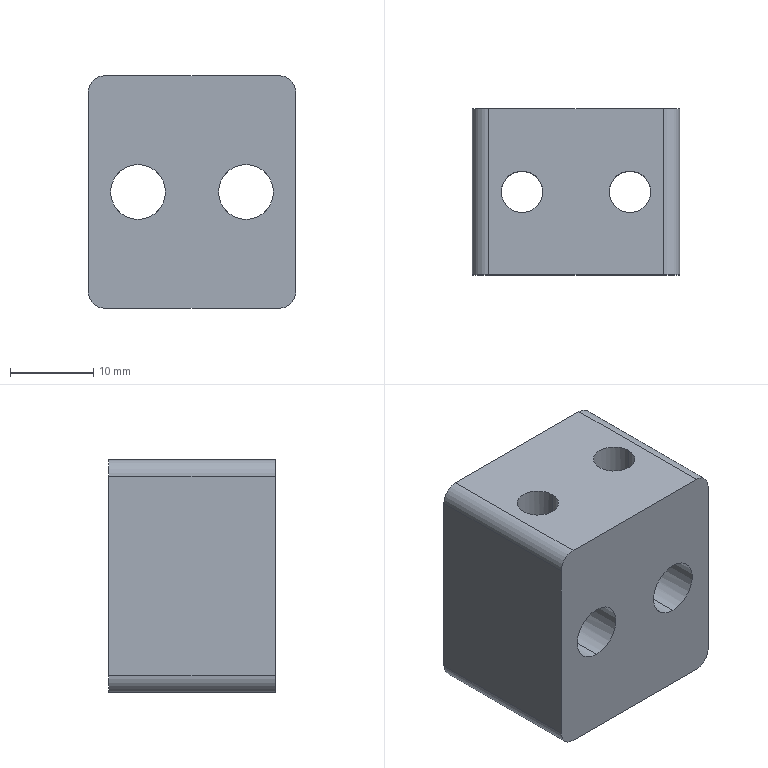Part | STEP file | 601-07-0069 | 1 solid | 28 faces | box 25 x 20 x 28 mm | volume 10875 mm3 | cylinder 20 | plane 8 | commonest cylinder face diameters 5 x8 4 x4 6.6 x4 11 x4